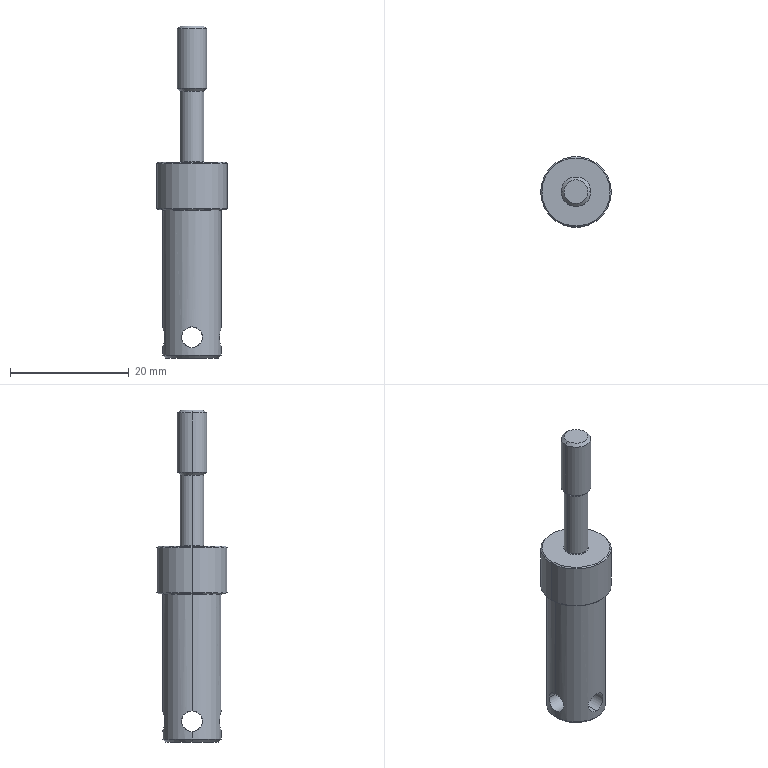Part | SolidWorks | features ICE 5, Chamfer 2, CirPattern 1, Extrusion 1, Fillet 1 | 1 solid | 34 faces | box 11.9 x 11.9 x 56 mm | volume 3013 mm3 | cylinder 16 | cone 10 | torus 4 | plane 4 | commonest cylinder face diameters 3.5 x8 4 x2 5 x2 9.9 x2 11.9 x2
STEP:
#1=CARTESIAN_POINT('',(-4.63,-1.75,-9.));
#2=VERTEX_POINT('',#1);
#3=CARTESIAN_POINT('',(-4.95,0.,-10.75));
#4=VERTEX_POINT('',#3);
#5=CARTESIAN_POINT('',(-4.63,-1.75,-9.));
#6=CARTESIAN_POINT('',(-4.63,-1.75,-9.115));
#7=CARTESIAN_POINT('',(-4.635,-1.738,-9.232));
#8=CARTESIAN_POINT('',(-4.652,-1.693,-9.457));
#9=CARTESIAN_POINT('',(-4.664,-1.66,-9.567));
#10=CARTESIAN_POINT('',(-4.694,-1.571,-9.78));
#11=CARTESIAN_POINT('',(-4.712,-1.517,-9.88));
#12=CARTESIAN_POINT('',(-4.751,-1.39,-10.069));
#13=CARTESIAN_POINT('',(-4.772,-1.317,-10.158));
#14=CARTESIAN_POINT('',(-4.814,-1.156,-10.319));
#15=CARTESIAN_POINT('',(-4.834,-1.069,-10.39));
#16=CARTESIAN_POINT('',(-4.872,-0.8798,-10.517));
#17=CARTESIAN_POINT('',(-4.89,-0.7775,-10.572));
#18=CARTESIAN_POINT('',(-4.933,-0.4616,-10.703));
#19=CARTESIAN_POINT('',(-4.95,-0.2297,-10.75));
#20=CARTESIAN_POINT('',(-4.95,0.,-10.75));
#21=B_SPLINE_CURVE_WITH_KNOTS('',3,(#5,#6,#7,#8,#9,#10,#11,#12,#13,#14,#15,#16,#17,#18,#19,#20),.UNSPECIFIED.,.F.,.F.,(4,2,2,2,2,2,2,4),(0.002759,0.003104,0.003448,0.003793,0.004138,0.004482,0.004827,0.005516),.UNSPECIFIED.);
#22=EDGE_CURVE('',#2,#4,#21,.T.);
#23=ORIENTED_EDGE('',*,*,#22,.F.);
#24=CARTESIAN_POINT('',(-1.75,-1.75,-9.));
#25=VERTEX_POINT('',#24);
#26=CARTESIAN_POINT('',(-8.5,-1.75,-9.));
#27=DIRECTION('',(1.,0.,0.));
#28=VECTOR('',#27,1000.);
#29=LINE('',#26,#28);
#30=EDGE_CURVE('',#2,#25,#29,.T.);
#31=ORIENTED_EDGE('',*,*,#30,.T.);
#32=CARTESIAN_POINT('',(0.,0.,-10.75));
#33=VERTEX_POINT('',#32);
#34=CARTESIAN_POINT('',(0.,0.,-10.75));
#35=CARTESIAN_POINT('',(-1.025,-1.025,-10.75));
#36=CARTESIAN_POINT('',(-1.75,-1.75,-10.025));
#37=CARTESIAN_POINT('',(-1.75,-1.75,-9.));
#38=(BOUNDED_CURVE()B_SPLINE_CURVE(3,(#34,#35,#36,#37),.UNSPECIFIED.,.F.,.F.)B_SPLINE_CURVE_WITH_KNOTS((4,4),(1.571,3.142),.UNSPECIFIED.)CURVE()GEOMETRIC_REPRESENTATION_ITEM()RATIONAL_B_SPLINE_CURVE((1.,0.8047,0.8047,1.))REPRESENTATION_ITEM(''));
#39=EDGE_CURVE('',#33,#25,#38,.T.);
#40=ORIENTED_EDGE('',*,*,#39,.F.);
#41=CARTESIAN_POINT('',(-1.75,1.75,-9.));
#42=VERTEX_POINT('',#41);
#43=CARTESIAN_POINT('',(-1.75,1.75,-9.));
#44=CARTESIAN_POINT('',(-1.75,1.75,-10.025));
#45=CARTESIAN_POINT('',(-1.025,1.025,-10.75));
#46=CARTESIAN_POINT('',(0.,0.,-10.75));
#47=(BOUNDED_CURVE()B_SPLINE_CURVE(3,(#43,#44,#45,#46),.UNSPECIFIED.,.F.,.F.)B_SPLINE_CURVE_WITH_KNOTS((4,4),(0.,1.571),.UNSPECIFIED.)CURVE()GEOMETRIC_REPRESENTATION_ITEM()RATIONAL_B_SPLINE_CURVE((1.,0.8047,0.8047,1.))REPRESENTATION_ITEM(''));
#48=EDGE_CURVE('',#42,#33,#47,.T.);
#49=ORIENTED_EDGE('',*,*,#48,.F.);
#50=CARTESIAN_POINT('',(-4.63,1.75,-9.));
#51=VERTEX_POINT('',#50);
#52=CARTESIAN_POINT('',(-8.5,1.75,-9.));
#53=DIRECTION('',(1.,0.,0.));
#54=VECTOR('',#53,1000.);
#55=LINE('',#52,#54);
#56=EDGE_CURVE('',#51,#42,#55,.T.);
#57=ORIENTED_EDGE('',*,*,#56,.F.);
#58=CARTESIAN_POINT('',(-4.95,0.,-10.75));
#59=CARTESIAN_POINT('',(-4.95,0.2297,-10.75));
#60=CARTESIAN_POINT('',(-4.933,0.4615,-10.704));
#61=CARTESIAN_POINT('',(-4.89,0.7784,-10.572));
#62=CARTESIAN_POINT('',(-4.872,0.8807,-10.517));
#63=CARTESIAN_POINT('',(-4.834,1.069,-10.39));
#64=CARTESIAN_POINT('',(-4.814,1.157,-10.318));
#65=CARTESIAN_POINT('',(-4.751,1.399,-10.075));
#66=CARTESIAN_POINT('',(-4.709,1.527,-9.885));
#67=CARTESIAN_POINT('',(-4.664,1.66,-9.566));
#68=CARTESIAN_POINT('',(-4.651,1.693,-9.457));
#69=CARTESIAN_POINT('',(-4.635,1.738,-9.232));
#70=CARTESIAN_POINT('',(-4.63,1.75,-9.115));
#71=CARTESIAN_POINT('',(-4.63,1.75,-9.));
#72=B_SPLINE_CURVE_WITH_KNOTS('',3,(#58,#59,#60,#61,#62,#63,#64,#65,#66,#67,#68,#69,#70,#71),.UNSPECIFIED.,.F.,.F.,(4,2,2,2,2,2,4),(0.005516,0.006206,0.00655,0.006895,0.007584,0.007929,0.008273),.UNSPECIFIED.);
#73=EDGE_CURVE('',#4,#51,#72,.T.);
#74=ORIENTED_EDGE('',*,*,#73,.F.);
#75=EDGE_LOOP('',(#23,#31,#40,#49,#57,#74));
#76=FACE_OUTER_BOUND('',#75,.T.);
#77=CARTESIAN_POINT('',(-8.5,0.,-9.));
#78=DIRECTION('',(1.,0.,0.));
#79=DIRECTION('',(0.,1.,0.));
#80=AXIS2_PLACEMENT_3D('',#77,#78,#79);
#81=CYLINDRICAL_SURFACE('',#80,1.75);
#82=ADVANCED_FACE('',(#76),#81,.F.);
#83=CARTESIAN_POINT('',(1.75,-1.75,-9.));
#84=VERTEX_POINT('',#83);
#85=CARTESIAN_POINT('',(1.75,-1.75,-9.));
#86=CARTESIAN_POINT('',(1.75,-1.75,-10.025));
#87=CARTESIAN_POINT('',(1.025,-1.025,-10.75));
#88=CARTESIAN_POINT('',(0.,0.,-10.75));
#89=(BOUNDED_CURVE()B_SPLINE_CURVE(3,(#85,#86,#87,#88),.UNSPECIFIED.,.F.,.F.)B_SPLINE_CURVE_WITH_KNOTS((4,4),(3.142,4.712),.UNSPECIFIED.)CURVE()GEOMETRIC_REPRESENTATION_ITEM()RATIONAL_B_SPLINE_CURVE((1.,0.8047,0.8047,1.))REPRESENTATION_ITEM(''));
#90=EDGE_CURVE('',#84,#33,#89,.T.);
#91=ORIENTED_EDGE('',*,*,#90,.F.);
#92=CARTESIAN_POINT('',(4.63,-1.75,-9.));
#93=VERTEX_POINT('',#92);
#94=CARTESIAN_POINT('',(-8.5,-1.75,-9.));
#95=DIRECTION('',(1.,0.,0.));
#96=VECTOR('',#95,1000.);
#97=LINE('',#94,#96);
#98=EDGE_CURVE('',#84,#93,#97,.T.);
#99=ORIENTED_EDGE('',*,*,#98,.T.);
#100=CARTESIAN_POINT('',(4.95,0.,-10.75));
#101=VERTEX_POINT('',#100);
#102=CARTESIAN_POINT('',(4.95,0.,-10.75));
#103=CARTESIAN_POINT('',(4.95,-0.1152,-10.75));
#104=CARTESIAN_POINT('',(4.946,-0.2322,-10.738));
#105=CARTESIAN_POINT('',(4.93,-0.4574,-10.693));
#106=CARTESIAN_POINT('',(4.919,-0.567,-10.66));
#107=CARTESIAN_POINT('',(4.889,-0.7801,-10.571));
#108=CARTESIAN_POINT('',(4.872,-0.8808,-10.516));
#109=CARTESIAN_POINT('',(4.834,-1.069,-10.39));
#110=CARTESIAN_POINT('',(4.813,-1.158,-10.317));
#111=CARTESIAN_POINT('',(4.772,-1.319,-10.156));
#112=CARTESIAN_POINT('',(4.751,-1.391,-10.068));
#113=CARTESIAN_POINT('',(4.712,-1.517,-9.879));
#114=CARTESIAN_POINT('',(4.694,-1.572,-9.777));
#115=CARTESIAN_POINT('',(4.649,-1.703,-9.462));
#116=CARTESIAN_POINT('',(4.63,-1.75,-9.23));
#117=CARTESIAN_POINT('',(4.63,-1.75,-9.));
#118=B_SPLINE_CURVE_WITH_KNOTS('',3,(#102,#103,#104,#105,#106,#107,#108,#109,#110,#111,#112,#113,#114,#115,#116,#117),.UNSPECIFIED.,.F.,.F.,(4,2,2,2,2,2,2,4),(0.002759,0.003104,0.003448,0.003793,0.004137,0.004482,0.004827,0.005516),.UNSPECIFIED.);
#119=EDGE_CURVE('',#101,#93,#118,.T.);
#120=ORIENTED_EDGE('',*,*,#119,.F.);
#121=CARTESIAN_POINT('',(4.63,1.75,-9.));
#122=VERTEX_POINT('',#121);
#123=CARTESIAN_POINT('',(4.63,1.75,-9.));
#124=CARTESIAN_POINT('',(4.63,1.75,-9.117));
#125=CARTESIAN_POINT('',(4.635,1.738,-9.231));
#126=CARTESIAN_POINT('',(4.651,1.693,-9.456));
#127=CARTESIAN_POINT('',(4.664,1.659,-9.568));
#128=CARTESIAN_POINT('',(4.694,1.571,-9.779));
#129=CARTESIAN_POINT('',(4.712,1.517,-9.879));
#130=CARTESIAN_POINT('',(4.751,1.39,-10.069));
#131=CARTESIAN_POINT('',(4.772,1.317,-10.158));
#132=CARTESIAN_POINT('',(4.834,1.077,-10.398));
#133=CARTESIAN_POINT('',(4.875,0.883,-10.528));
#134=CARTESIAN_POINT('',(4.919,0.5674,-10.659));
#135=CARTESIAN_POINT('',(4.93,0.456,-10.693));
#136=CARTESIAN_POINT('',(4.946,0.2295,-10.739));
#137=CARTESIAN_POINT('',(4.95,0.1153,-10.75));
#138=CARTESIAN_POINT('',(4.95,0.,-10.75));
#139=B_SPLINE_CURVE_WITH_KNOTS('',3,(#123,#124,#125,#126,#127,#128,#129,#130,#131,#132,#133,#134,#135,#136,#137,#138),.UNSPECIFIED.,.F.,.F.,(4,2,2,2,2,2,2,4),(0.,0.0003449,0.0006897,0.001035,0.001379,0.002069,0.002414,0.002759),.UNSPECIFIED.);
#140=EDGE_CURVE('',#122,#101,#139,.T.);
#141=ORIENTED_EDGE('',*,*,#140,.F.);
#142=CARTESIAN_POINT('',(1.75,1.75,-9.));
#143=VERTEX_POINT('',#142);
#144=CARTESIAN_POINT('',(-8.5,1.75,-9.));
#145=DIRECTION('',(1.,0.,0.));
#146=VECTOR('',#145,1000.);
#147=LINE('',#144,#146);
#148=EDGE_CURVE('',#143,#122,#147,.T.);
#149=ORIENTED_EDGE('',*,*,#148,.F.);
#150=CARTESIAN_POINT('',(0.,0.,-10.75));
#151=CARTESIAN_POINT('',(1.025,1.025,-10.75));
#152=CARTESIAN_POINT('',(1.75,1.75,-10.025));
#153=CARTESIAN_POINT('',(1.75,1.75,-9.));
#154=(BOUNDED_CURVE()B_SPLINE_CURVE(3,(#150,#151,#152,#153),.UNSPECIFIED.,.F.,.F.)B_SPLINE_CURVE_WITH_KNOTS((4,4),(4.712,6.283),.UNSPECIFIED.)CURVE()GEOMETRIC_REPRESENTATION_ITEM()RATIONAL_B_SPLINE_CURVE((1.,0.8047,0.8047,1.))REPRESENTATION_ITEM(''));
#155=EDGE_CURVE('',#33,#143,#154,.T.);
#156=ORIENTED_EDGE('',*,*,#155,.F.);
#157=EDGE_LOOP('',(#91,#99,#120,#141,#149,#156));
#158=FACE_OUTER_BOUND('',#157,.T.);
#159=CARTESIAN_POINT('',(-8.5,0.,-9.));
#160=DIRECTION('',(1.,0.,0.));
#161=DIRECTION('',(0.,1.,0.));
#162=AXIS2_PLACEMENT_3D('',#159,#160,#161);
#163=CYLINDRICAL_SURFACE('',#162,1.75);
#164=ADVANCED_FACE('',(#158),#163,.F.);
#165=CARTESIAN_POINT('',(0.,-4.95,-10.75));
#166=VERTEX_POINT('',#165);
#167=CARTESIAN_POINT('',(0.,-4.95,-7.25));
#168=VERTEX_POINT('',#167);
#169=CARTESIAN_POINT('',(0.,-4.95,-10.75));
#170=CARTESIAN_POINT('',(-0.2297,-4.95,-10.75));
#171=CARTESIAN_POINT('',(-0.4616,-4.933,-10.703));
#172=CARTESIAN_POINT('',(-0.7785,-4.89,-10.571));
#173=CARTESIAN_POINT('',(-0.8808,-4.872,-10.516));
#174=CARTESIAN_POINT('',(-1.07,-4.834,-10.39));
#175=CARTESIAN_POINT('',(-1.157,-4.814,-10.318));
#176=CARTESIAN_POINT('',(-1.4,-4.751,-10.075));
#177=CARTESIAN_POINT('',(-1.528,-4.709,-9.884));
#178=CARTESIAN_POINT('',(-1.66,-4.664,-9.566));
#179=CARTESIAN_POINT('',(-1.693,-4.651,-9.457));
#180=CARTESIAN_POINT('',(-1.738,-4.635,-9.232));
#181=CARTESIAN_POINT('',(-1.75,-4.63,-9.115));
#182=CARTESIAN_POINT('',(-1.75,-4.63,-8.884));
#183=CARTESIAN_POINT('',(-1.739,-4.635,-8.77));
#184=CARTESIAN_POINT('',(-1.693,-4.651,-8.543));
#185=CARTESIAN_POINT('',(-1.659,-4.664,-8.432));
#186=CARTESIAN_POINT('',(-1.528,-4.709,-8.116));
#187=CARTESIAN_POINT('',(-1.398,-4.751,-7.923));
#188=CARTESIAN_POINT('',(-1.157,-4.814,-7.682));
#189=CARTESIAN_POINT('',(-1.068,-4.834,-7.609));
#190=CARTESIAN_POINT('',(-0.8791,-4.872,-7.483));
#191=CARTESIAN_POINT('',(-0.779,-4.889,-7.429));
#192=CARTESIAN_POINT('',(-0.567,-4.919,-7.34));
#193=CARTESIAN_POINT('',(-0.4557,-4.93,-7.306));
#194=CARTESIAN_POINT('',(-0.2311,-4.946,-7.262));
#195=CARTESIAN_POINT('',(-0.1166,-4.95,-7.25));
#196=CARTESIAN_POINT('',(0.,-4.95,-7.25));
#197=B_SPLINE_CURVE_WITH_KNOTS('',3,(#169,#170,#171,#172,#173,#174,#175,#176,#177,#178,#179,#180,#181,#182,#183,#184,#185,#186,#187,#188,#189,#190,#191,#192,#193,#194,#195,#196),.UNSPECIFIED.,.F.,.F.,(4,2,2,2,2,2,2,2,2,2,2,2,2,4),(0.005516,0.006206,0.00655,0.006895,0.007584,0.007929,0.008274,0.008618,0.008963,0.009652,0.009997,0.01034,0.01069,0.01103),.UNSPECIFIED.);
#198=EDGE_CURVE('',#166,#168,#197,.T.);
#199=ORIENTED_EDGE('',*,*,#198,.F.);
#200=CARTESIAN_POINT('',(0.,-8.5,-10.75));
#201=DIRECTION('',(0.,1.,0.));
#202=VECTOR('',#201,1000.);
#203=LINE('',#200,#202);
#204=EDGE_CURVE('',#166,#33,#203,.T.);
#205=ORIENTED_EDGE('',*,*,#204,.T.);
#206=ORIENTED_EDGE('',*,*,#39,.T.);
#207=CARTESIAN_POINT('',(0.,0.,-7.25));
#208=VERTEX_POINT('',#207);
#209=CARTESIAN_POINT('',(-1.75,-1.75,-9.));
#210=CARTESIAN_POINT('',(-1.75,-1.75,-7.975));
#211=CARTESIAN_POINT('',(-1.025,-1.025,-7.25));
#212=CARTESIAN_POINT('',(0.,0.,-7.25));
#213=(BOUNDED_CURVE()B_SPLINE_CURVE(3,(#209,#210,#211,#212),.UNSPECIFIED.,.F.,.F.)B_SPLINE_CURVE_WITH_KNOTS((4,4),(3.142,4.712),.UNSPECIFIED.)CURVE()GEOMETRIC_REPRESENTATION_ITEM()RATIONAL_B_SPLINE_CURVE((1.,0.8047,0.8047,1.))REPRESENTATION_ITEM(''));
#214=EDGE_CURVE('',#25,#208,#213,.T.);
#215=ORIENTED_EDGE('',*,*,#214,.T.);
#216=CARTESIAN_POINT('',(0.,-8.5,-7.25));
#217=DIRECTION('',(0.,1.,0.));
#218=VECTOR('',#217,1000.);
#219=LINE('',#216,#218);
#220=EDGE_CURVE('',#168,#208,#219,.T.);
#221=ORIENTED_EDGE('',*,*,#220,.F.);
#222=EDGE_LOOP('',(#199,#205,#206,#215,#221));
#223=FACE_OUTER_BOUND('',#222,.T.);
#224=CARTESIAN_POINT('',(0.,-8.5,-9.));
#225=DIRECTION('',(0.,1.,0.));
#226=DIRECTION('',(0.,0.,1.));
#227=AXIS2_PLACEMENT_3D('',#224,#225,#226);
#228=CYLINDRICAL_SURFACE('',#227,1.75);
#229=ADVANCED_FACE('',(#223),#228,.F.);
#230=CARTESIAN_POINT('',(-5.05,0.,12.5));
#231=VERTEX_POINT('',#230);
#232=CARTESIAN_POINT('',(5.05,0.,12.5));
#233=VERTEX_POINT('',#232);
#234=CARTESIAN_POINT('',(0.,0.,12.5));
#235=DIRECTION('',(0.,0.,1.));
#236=DIRECTION('',(1.,0.,0.));
#237=AXIS2_PLACEMENT_3D('',#234,#235,#236);
#238=CIRCLE('',#237,5.05);
#239=EDGE_CURVE('',#231,#233,#238,.T.);
#240=ORIENTED_EDGE('',*,*,#239,.F.);
#241=CARTESIAN_POINT('',(-4.95,0.,12.4));
#242=VERTEX_POINT('',#241);
#243=CARTESIAN_POINT('',(-5.05,0.,12.4));
#244=DIRECTION('',(0.,1.,0.));
#245=DIRECTION('',(-1.,0.,0.));
#246=AXIS2_PLACEMENT_3D('',#243,#244,#245);
#247=CIRCLE('',#246,0.1);
#248=EDGE_CURVE('',#231,#242,#247,.T.);
#249=ORIENTED_EDGE('',*,*,#248,.T.);
#250=CARTESIAN_POINT('',(4.95,0.,12.4));
#251=VERTEX_POINT('',#250);
#252=CARTESIAN_POINT('',(0.,0.,12.4));
#253=DIRECTION('',(0.,0.,-1.));
#254=DIRECTION('',(1.,0.,0.));
#255=AXIS2_PLACEMENT_3D('',#252,#253,#254);
#256=CIRCLE('',#255,4.95);
#257=EDGE_CURVE('',#251,#242,#256,.T.);
#258=ORIENTED_EDGE('',*,*,#257,.F.);
#259=CARTESIAN_POINT('',(5.05,0.,12.4));
#260=DIRECTION('',(0.,-1.,0.));
#261=DIRECTION('',(0.,0.,-1.));
#262=AXIS2_PLACEMENT_3D('',#259,#260,#261);
#263=CIRCLE('',#262,0.1);
#264=EDGE_CURVE('',#233,#251,#263,.T.);
#265=ORIENTED_EDGE('',*,*,#264,.F.);
#266=EDGE_LOOP('',(#240,#249,#258,#265));
#267=FACE_OUTER_BOUND('',#266,.T.);
#268=CARTESIAN_POINT('',(0.,0.,12.4));
#269=DIRECTION('',(0.,0.,1.));
#270=DIRECTION('',(1.,0.,0.));
#271=AXIS2_PLACEMENT_3D('',#268,#269,#270);
#272=TOROIDAL_SURFACE('',#271,5.05,0.1);
#273=ADVANCED_FACE('',(#267),#272,.F.);
#274=CARTESIAN_POINT('',(-2.,0.,20.6));
#275=VERTEX_POINT('',#274);
#276=CARTESIAN_POINT('',(2.,0.,20.6));
#277=VERTEX_POINT('',#276);
#278=CARTESIAN_POINT('',(0.,0.,20.6));
#279=DIRECTION('',(0.,0.,1.));
#280=DIRECTION('',(1.,0.,0.));
#281=AXIS2_PLACEMENT_3D('',#278,#279,#280);
#282=CIRCLE('',#281,2.);
#283=EDGE_CURVE('',#275,#277,#282,.T.);
#284=ORIENTED_EDGE('',*,*,#283,.F.);
#285=CARTESIAN_POINT('',(-2.1,0.,20.5));
#286=VERTEX_POINT('',#285);
#287=CARTESIAN_POINT('',(-2.1,0.,20.6));
#288=DIRECTION('',(0.,1.,0.));
#289=DIRECTION('',(-1.,0.,0.));
#290=AXIS2_PLACEMENT_3D('',#287,#288,#289);
#291=CIRCLE('',#290,0.1);
#292=EDGE_CURVE('',#275,#286,#291,.T.);
#293=ORIENTED_EDGE('',*,*,#292,.T.);
#294=CARTESIAN_POINT('',(2.1,0.,20.5));
#295=VERTEX_POINT('',#294);
#296=CARTESIAN_POINT('',(0.,0.,20.5));
#297=DIRECTION('',(0.,0.,-1.));
#298=DIRECTION('',(1.,0.,0.));
#299=AXIS2_PLACEMENT_3D('',#296,#297,#298);
#300=CIRCLE('',#299,2.1);
#301=EDGE_CURVE('',#295,#286,#300,.T.);
#302=ORIENTED_EDGE('',*,*,#301,.F.);
#303=CARTESIAN_POINT('',(2.1,0.,20.6));
#304=DIRECTION('',(0.,-1.,0.));
#305=DIRECTION('',(0.,0.,-1.));
#306=AXIS2_PLACEMENT_3D('',#303,#304,#305);
#307=CIRCLE('',#306,0.1);
#308=EDGE_CURVE('',#277,#295,#307,.T.);
#309=ORIENTED_EDGE('',*,*,#308,.F.);
#310=EDGE_LOOP('',(#284,#293,#302,#309));
#311=FACE_OUTER_BOUND('',#310,.T.);
#312=CARTESIAN_POINT('',(0.,0.,20.6));
#313=DIRECTION('',(0.,0.,1.));
#314=DIRECTION('',(1.,0.,0.));
#315=AXIS2_PLACEMENT_3D('',#312,#313,#314);
#316=TOROIDAL_SURFACE('',#315,2.1,0.1);
#317=ADVANCED_FACE('',(#311),#316,.F.);
#318=CARTESIAN_POINT('',(-5.75,0.,12.5));
#319=VERTEX_POINT('',#318);
#320=CARTESIAN_POINT('',(5.75,0.,12.5));
#321=VERTEX_POINT('',#320);
#322=CARTESIAN_POINT('',(0.,0.,12.5));
#323=DIRECTION('',(0.,0.,-1.));
#324=DIRECTION('',(1.,0.,0.));
#325=AXIS2_PLACEMENT_3D('',#322,#323,#324);
#326=CIRCLE('',#325,5.75);
#327=EDGE_CURVE('',#319,#321,#326,.T.);
#328=ORIENTED_EDGE('',*,*,#327,.F.);
#329=CARTESIAN_POINT('',(-5.95,0.,12.7));
#330=VERTEX_POINT('',#329);
#331=CARTESIAN_POINT('',(-5.95,0.,12.7));
#332=DIRECTION('',(-0.7071,0.,0.7071));
#333=VECTOR('',#332,1000.);
#334=LINE('',#331,#333);
#335=EDGE_CURVE('',#319,#330,#334,.T.);
#336=ORIENTED_EDGE('',*,*,#335,.T.);
#337=CARTESIAN_POINT('',(5.95,0.,12.7));
#338=VERTEX_POINT('',#337);
#339=CARTESIAN_POINT('',(0.,0.,12.7));
#340=DIRECTION('',(0.,0.,1.));
#341=DIRECTION('',(1.,0.,0.));
#342=AXIS2_PLACEMENT_3D('',#339,#340,#341);
#343=CIRCLE('',#342,5.95);
#344=EDGE_CURVE('',#338,#330,#343,.T.);
#345=ORIENTED_EDGE('',*,*,#344,.F.);
#346=CARTESIAN_POINT('',(5.95,0.,12.7));
#347=DIRECTION('',(0.7071,0.,0.7071));
#348=VECTOR('',#347,1000.);
#349=LINE('',#346,#348);
#350=EDGE_CURVE('',#321,#338,#349,.T.);
#351=ORIENTED_EDGE('',*,*,#350,.F.);
#352=EDGE_LOOP('',(#328,#336,#345,#351));
#353=FACE_OUTER_BOUND('',#352,.T.);
#354=CARTESIAN_POINT('',(0.,0.,12.7));
#355=DIRECTION('',(0.,0.,1.));
#356=DIRECTION('',(1.,0.,0.));
#357=AXIS2_PLACEMENT_3D('',#354,#355,#356);
#358=CONICAL_SURFACE('',#357,5.95,0.7854);
#359=ADVANCED_FACE('',(#353),#358,.T.);
#360=CARTESIAN_POINT('',(5.75,0.,20.5));
#361=VERTEX_POINT('',#360);
#362=CARTESIAN_POINT('',(-5.75,0.,20.5));
#363=VERTEX_POINT('',#362);
#364=CARTESIAN_POINT('',(0.,0.,20.5));
#365=DIRECTION('',(0.,0.,1.));
#366=DIRECTION('',(1.,0.,0.));
#367=AXIS2_PLACEMENT_3D('',#364,#365,#366);
#368=CIRCLE('',#367,5.75);
#369=EDGE_CURVE('',#361,#363,#368,.T.);
#370=ORIENTED_EDGE('',*,*,#369,.F.);
#371=CARTESIAN_POINT('',(5.95,0.,20.3));
#372=VERTEX_POINT('',#371);
#373=CARTESIAN_POINT('',(5.75,0.,20.5));
#374=DIRECTION('',(0.7071,0.,-0.7071));
#375=VECTOR('',#374,1000.);
#376=LINE('',#373,#375);
#377=EDGE_CURVE('',#361,#372,#376,.T.);
#378=ORIENTED_EDGE('',*,*,#377,.T.);
#379=CARTESIAN_POINT('',(-5.95,0.,20.3));
#380=VERTEX_POINT('',#379);
#381=CARTESIAN_POINT('',(0.,0.,20.3));
#382=DIRECTION('',(0.,0.,-1.));
#383=DIRECTION('',(1.,0.,0.));
#384=AXIS2_PLACEMENT_3D('',#381,#382,#383);
#385=CIRCLE('',#384,5.95);
#386=EDGE_CURVE('',#380,#372,#385,.T.);
#387=ORIENTED_EDGE('',*,*,#386,.F.);
#388=CARTESIAN_POINT('',(-5.75,0.,20.5));
#389=DIRECTION('',(-0.7071,0.,-0.7071));
#390=VECTOR('',#389,1000.);
#391=LINE('',#388,#390);
#392=EDGE_CURVE('',#363,#380,#391,.T.);
#393=ORIENTED_EDGE('',*,*,#392,.F.);
#394=EDGE_LOOP('',(#370,#378,#387,#393));
#395=FACE_OUTER_BOUND('',#394,.T.);
#396=CARTESIAN_POINT('',(0.,0.,20.5));
#397=DIRECTION('',(0.,0.,-1.));
#398=DIRECTION('',(-1.,0.,0.));
#399=AXIS2_PLACEMENT_3D('',#396,#397,#398);
#400=CONICAL_SURFACE('',#399,5.75,0.7854);
#401=ADVANCED_FACE('',(#395),#400,.T.);
#402=CARTESIAN_POINT('',(-4.45,0.,-12.5));
#403=VERTEX_POINT('',#402);
#404=CARTESIAN_POINT('',(4.45,0.,-12.5));
#405=VERTEX_POINT('',#404);
#406=CARTESIAN_POINT('',(0.,0.,-12.5));
#407=DIRECTION('',(0.,0.,-1.));
#408=DIRECTION('',(1.,0.,0.));
#409=AXIS2_PLACEMENT_3D('',#406,#407,#408);
#410=CIRCLE('',#409,4.45);
#411=EDGE_CURVE('',#403,#405,#410,.T.);
#412=ORIENTED_EDGE('',*,*,#411,.F.);
#413=CARTESIAN_POINT('',(-4.95,0.,-12.));
#414=VERTEX_POINT('',#413);
#415=CARTESIAN_POINT('',(-4.95,0.,-12.));
#416=DIRECTION('',(-0.7071,0.,0.7071));
#417=VECTOR('',#416,1000.);
#418=LINE('',#415,#417);
#419=EDGE_CURVE('',#403,#414,#418,.T.);
#420=ORIENTED_EDGE('',*,*,#419,.T.);
#421=CARTESIAN_POINT('',(4.95,0.,-12.));
#422=VERTEX_POINT('',#421);
#423=CARTESIAN_POINT('',(0.,0.,-12.));
#424=DIRECTION('',(0.,0.,1.));
#425=DIRECTION('',(1.,0.,0.));
#426=AXIS2_PLACEMENT_3D('',#423,#424,#425);
#427=CIRCLE('',#426,4.95);
#428=EDGE_CURVE('',#422,#414,#427,.T.);
#429=ORIENTED_EDGE('',*,*,#428,.F.);
#430=CARTESIAN_POINT('',(4.95,0.,-12.));
#431=DIRECTION('',(0.7071,0.,0.7071));
#432=VECTOR('',#431,1000.);
#433=LINE('',#430,#432);
#434=EDGE_CURVE('',#405,#422,#433,.T.);
#435=ORIENTED_EDGE('',*,*,#434,.F.);
#436=EDGE_LOOP('',(#412,#420,#429,#435));
#437=FACE_OUTER_BOUND('',#436,.T.);
#438=CARTESIAN_POINT('',(0.,0.,-12.));
#439=DIRECTION('',(0.,0.,1.));
#440=DIRECTION('',(1.,0.,0.));
#441=AXIS2_PLACEMENT_3D('',#438,#439,#440);
#442=CONICAL_SURFACE('',#441,4.95,0.7854);
#443=ADVANCED_FACE('',(#437),#442,.T.);
#444=CARTESIAN_POINT('',(2.,0.,43.5));
#445=VERTEX_POINT('',#444);
#446=CARTESIAN_POINT('',(-2.,0.,43.5));
#447=VERTEX_POINT('',#446);
#448=CARTESIAN_POINT('',(0.,0.,43.5));
#449=DIRECTION('',(0.,0.,1.));
#450=DIRECTION('',(1.,0.,0.));
#451=AXIS2_PLACEMENT_3D('',#448,#449,#450);
#452=CIRCLE('',#451,2.);
#453=EDGE_CURVE('',#445,#447,#452,.T.);
#454=ORIENTED_EDGE('',*,*,#453,.F.);
#455=CARTESIAN_POINT('',(2.5,0.,43.));
#456=VERTEX_POINT('',#455);
#457=CARTESIAN_POINT('',(2.,0.,43.5));
#458=DIRECTION('',(0.7071,0.,-0.7071));
#459=VECTOR('',#458,1000.);
#460=LINE('',#457,#459);
#461=EDGE_CURVE('',#445,#456,#460,.T.);
#462=ORIENTED_EDGE('',*,*,#461,.T.);
#463=CARTESIAN_POINT('',(-2.5,0.,43.));
#464=VERTEX_POINT('',#463);
#465=CARTESIAN_POINT('',(0.,0.,43.));
#466=DIRECTION('',(0.,0.,-1.));
#467=DIRECTION('',(1.,0.,0.));
#468=AXIS2_PLACEMENT_3D('',#465,#466,#467);
#469=CIRCLE('',#468,2.5);
#470=EDGE_CURVE('',#464,#456,#469,.T.);
#471=ORIENTED_EDGE('',*,*,#470,.F.);
#472=CARTESIAN_POINT('',(-2.,0.,43.5));
#473=DIRECTION('',(-0.7071,0.,-0.7071));
#474=VECTOR('',#473,1000.);
#475=LINE('',#472,#474);
#476=EDGE_CURVE('',#447,#464,#475,.T.);
#477=ORIENTED_EDGE('',*,*,#476,.F.);
#478=EDGE_LOOP('',(#454,#462,#471,#477));
#479=FACE_OUTER_BOUND('',#478,.T.);
#480=CARTESIAN_POINT('',(0.,0.,43.5));
#481=DIRECTION('',(0.,0.,-1.));
#482=DIRECTION('',(-1.,0.,0.));
#483=AXIS2_PLACEMENT_3D('',#480,#481,#482);
#484=CONICAL_SURFACE('',#483,2.,0.7854);
#485=ADVANCED_FACE('',(#479),#484,.T.);
#486=CARTESIAN_POINT('',(2.,0.,32.5));
#487=VERTEX_POINT('',#486);
#488=CARTESIAN_POINT('',(-2.,0.,32.5));
#489=VERTEX_POINT('',#488);
#490=CARTESIAN_POINT('',(0.,0.,32.5));
#491=DIRECTION('',(0.,0.,1.));
#492=DIRECTION('',(1.,0.,0.));
#493=AXIS2_PLACEMENT_3D('',#490,#491,#492);
#494=CIRCLE('',#493,2.);
#495=EDGE_CURVE('',#487,#489,#494,.T.);
#496=ORIENTED_EDGE('',*,*,#495,.T.);
#497=CARTESIAN_POINT('',(-2.5,0.,33.));
#498=VERTEX_POINT('',#497);
#499=CARTESIAN_POINT('',(-2.5,0.,33.));
#500=DIRECTION('',(-0.7071,0.,0.7071));
#501=VECTOR('',#500,1000.);
#502=LINE('',#499,#501);
#503=EDGE_CURVE('',#489,#498,#502,.T.);
#504=ORIENTED_EDGE('',*,*,#503,.T.);
#505=CARTESIAN_POINT('',(2.5,0.,33.));
#506=VERTEX_POINT('',#505);
#507=CARTESIAN_POINT('',(0.,0.,33.));
#508=DIRECTION('',(0.,0.,1.));
#509=DIRECTION('',(1.,0.,0.));
#510=AXIS2_PLACEMENT_3D('',#507,#508,#509);
#511=CIRCLE('',#510,2.5);
#512=EDGE_CURVE('',#506,#498,#511,.T.);
#513=ORIENTED_EDGE('',*,*,#512,.F.);
#514=CARTESIAN_POINT('',(2.5,0.,33.));
#515=DIRECTION('',(0.7071,0.,0.7071));
#516=VECTOR('',#515,1000.);
#517=LINE('',#514,#516);
#518=EDGE_CURVE('',#487,#506,#517,.T.);
#519=ORIENTED_EDGE('',*,*,#518,.F.);
#520=EDGE_LOOP('',(#496,#504,#513,#519));
#521=FACE_OUTER_BOUND('',#520,.T.);
#522=CARTESIAN_POINT('',(0.,0.,33.));
#523=DIRECTION('',(0.,0.,1.));
#524=DIRECTION('',(1.,0.,0.));
#525=AXIS2_PLACEMENT_3D('',#522,#523,#524);
#526=CONICAL_SURFACE('',#525,2.5,0.7854);
#527=ADVANCED_FACE('',(#521),#526,.T.);
#528=ORIENTED_EDGE('',*,*,#470,.T.);
#529=CARTESIAN_POINT('',(2.5,0.,43.5));
#530=DIRECTION('',(0.,0.,-1.));
#531=VECTOR('',#530,1000.);
#532=LINE('',#529,#531);
#533=EDGE_CURVE('',#456,#506,#532,.T.);
#534=ORIENTED_EDGE('',*,*,#533,.T.);
#535=ORIENTED_EDGE('',*,*,#512,.T.);
#536=CARTESIAN_POINT('',(-2.5,0.,43.5));
#537=DIRECTION('',(0.,0.,-1.));
#538=VECTOR('',#537,1000.);
#539=LINE('',#536,#538);
#540=EDGE_CURVE('',#464,#498,#539,.T.);
#541=ORIENTED_EDGE('',*,*,#540,.F.);
#542=EDGE_LOOP('',(#528,#534,#535,#541));
#543=FACE_OUTER_BOUND('',#542,.T.);
#544=CARTESIAN_POINT('',(0.,0.,43.5));
#545=DIRECTION('',(0.,0.,-1.));
#546=DIRECTION('',(-1.,0.,0.));
#547=AXIS2_PLACEMENT_3D('',#544,#545,#546);
#548=CYLINDRICAL_SURFACE('',#547,2.5);
#549=ADVANCED_FACE('',(#543),#548,.T.);
#550=ORIENTED_EDGE('',*,*,#495,.F.);
#551=CARTESIAN_POINT('',(2.,0.,32.5));
#552=DIRECTION('',(0.,0.,-1.));
#553=VECTOR('',#552,1000.);
#554=LINE('',#551,#553);
#555=EDGE_CURVE('',#487,#277,#554,.T.);
#556=ORIENTED_EDGE('',*,*,#555,.T.);
#557=CARTESIAN_POINT('',(0.,0.,20.6));
#558=DIRECTION('',(0.,0.,1.));
#559=DIRECTION('',(1.,0.,0.));
#560=AXIS2_PLACEMENT_3D('',#557,#558,#559);
#561=CIRCLE('',#560,2.);
#562=EDGE_CURVE('',#277,#275,#561,.T.);
#563=ORIENTED_EDGE('',*,*,#562,.T.);
#564=CARTESIAN_POINT('',(-2.,0.,32.5));
#565=DIRECTION('',(0.,0.,-1.));
#566=VECTOR('',#565,1000.);
#567=LINE('',#564,#566);
#568=EDGE_CURVE('',#489,#275,#567,.T.);
#569=ORIENTED_EDGE('',*,*,#568,.F.);
#570=EDGE_LOOP('',(#550,#556,#563,#569));
#571=FACE_OUTER_BOUND('',#570,.T.);
#572=CARTESIAN_POINT('',(0.,0.,32.5));
#573=DIRECTION('',(0.,0.,-1.));
#574=DIRECTION('',(-1.,0.,0.));
#575=AXIS2_PLACEMENT_3D('',#572,#573,#574);
#576=CYLINDRICAL_SURFACE('',#575,2.);
#577=ADVANCED_FACE('',(#571),#576,.T.);
#578=ORIENTED_EDGE('',*,*,#386,.T.);
#579=CARTESIAN_POINT('',(5.95,0.,20.5));
#580=DIRECTION('',(0.,0.,-1.));
#581=VECTOR('',#580,1000.);
#582=LINE('',#579,#581);
#583=EDGE_CURVE('',#372,#338,#582,.T.);
#584=ORIENTED_EDGE('',*,*,#583,.T.);
#585=ORIENTED_EDGE('',*,*,#344,.T.);
#586=CARTESIAN_POINT('',(-5.95,0.,20.5));
#587=DIRECTION('',(0.,0.,-1.));
#588=VECTOR('',#587,1000.);
#589=LINE('',#586,#588);
#590=EDGE_CURVE('',#380,#330,#589,.T.);
#591=ORIENTED_EDGE('',*,*,#590,.F.);
#592=EDGE_LOOP('',(#578,#584,#585,#591));
#593=FACE_OUTER_BOUND('',#592,.T.);
#594=CARTESIAN_POINT('',(0.,0.,20.5));
#595=DIRECTION('',(0.,0.,-1.));
#596=DIRECTION('',(-1.,0.,0.));
#597=AXIS2_PLACEMENT_3D('',#594,#595,#596);
#598=CYLINDRICAL_SURFACE('',#597,5.95);
#599=ADVANCED_FACE('',(#593),#598,.T.);
#600=CARTESIAN_POINT('',(0.,4.95,-7.25));
#601=VERTEX_POINT('',#600);
#602=CARTESIAN_POINT('',(0.,4.95,-10.75));
#603=VERTEX_POINT('',#602);
#604=CARTESIAN_POINT('',(0.,4.95,-7.25));
#605=CARTESIAN_POINT('',(-0.1166,4.95,-7.25));
#606=CARTESIAN_POINT('',(-0.2312,4.946,-7.262));
#607=CARTESIAN_POINT('',(-0.4562,4.93,-7.307));
#608=CARTESIAN_POINT('',(-0.5678,4.918,-7.341));
#609=CARTESIAN_POINT('',(-0.7794,4.889,-7.429));
#610=CARTESIAN_POINT('',(-0.8796,4.872,-7.483));
#611=CARTESIAN_POINT('',(-1.069,4.834,-7.61));
#612=CARTESIAN_POINT('',(-1.158,4.813,-7.683));
#613=CARTESIAN_POINT('',(-1.398,4.751,-7.923));
#614=CARTESIAN_POINT('',(-1.528,4.709,-8.117));
#615=CARTESIAN_POINT('',(-1.659,4.664,-8.432));
#616=CARTESIAN_POINT('',(-1.693,4.651,-8.543));
#617=CARTESIAN_POINT('',(-1.739,4.635,-8.77));
#618=CARTESIAN_POINT('',(-1.75,4.63,-8.884));
#619=CARTESIAN_POINT('',(-1.75,4.63,-9.114));
#620=CARTESIAN_POINT('',(-1.738,4.635,-9.231));
#621=CARTESIAN_POINT('',(-1.693,4.651,-9.457));
#622=CARTESIAN_POINT('',(-1.66,4.664,-9.566));
#623=CARTESIAN_POINT('',(-1.571,4.694,-9.779));
#624=CARTESIAN_POINT('',(-1.517,4.712,-9.88));
#625=CARTESIAN_POINT('',(-1.391,4.751,-10.068));
#626=CARTESIAN_POINT('',(-1.317,4.772,-10.158));
#627=CARTESIAN_POINT('',(-1.157,4.814,-10.318));
#628=CARTESIAN_POINT('',(-1.069,4.834,-10.39));
#629=CARTESIAN_POINT('',(-0.88,4.872,-10.517));
#630=CARTESIAN_POINT('',(-0.7777,4.89,-10.572));
#631=CARTESIAN_POINT('',(-0.4617,4.933,-10.703));
#632=CARTESIAN_POINT('',(-0.2298,4.95,-10.75));
#633=CARTESIAN_POINT('',(0.,4.95,-10.75));
#634=B_SPLINE_CURVE_WITH_KNOTS('',3,(#604,#605,#606,#607,#608,#609,#610,#611,#612,#613,#614,#615,#616,#617,#618,#619,#620,#621,#622,#623,#624,#625,#626,#627,#628,#629,#630,#631,#632,#633),.UNSPECIFIED.,.F.,.F.,(4,2,2,2,2,2,2,2,2,2,2,2,2,2,4),(0.,0.0003448,0.0006895,0.001034,0.001379,0.002069,0.002413,0.002758,0.003103,0.003448,0.003792,0.004137,0.004482,0.004827,0.005516),.UNSPECIFIED.);
#635=EDGE_CURVE('',#601,#603,#634,.T.);
#636=ORIENTED_EDGE('',*,*,#635,.T.);
#637=CARTESIAN_POINT('',(0.,4.95,-10.75));
#638=CARTESIAN_POINT('',(0.2297,4.95,-10.75));
#639=CARTESIAN_POINT('',(0.4616,4.933,-10.703));
#640=CARTESIAN_POINT('',(0.7785,4.89,-10.571));
#641=CARTESIAN_POINT('',(0.8808,4.872,-10.516));
#642=CARTESIAN_POINT('',(1.07,4.834,-10.39));
#643=CARTESIAN_POINT('',(1.157,4.814,-10.318));
#644=CARTESIAN_POINT('',(1.4,4.751,-10.075));
#645=CARTESIAN_POINT('',(1.528,4.709,-9.884));
#646=CARTESIAN_POINT('',(1.66,4.664,-9.566));
#647=CARTESIAN_POINT('',(1.693,4.651,-9.457));
#648=CARTESIAN_POINT('',(1.738,4.635,-9.232));
#649=CARTESIAN_POINT('',(1.75,4.63,-9.115));
#650=CARTESIAN_POINT('',(1.75,4.63,-8.884));
#651=CARTESIAN_POINT('',(1.739,4.635,-8.77));
#652=CARTESIAN_POINT('',(1.693,4.651,-8.543));
#653=CARTESIAN_POINT('',(1.659,4.664,-8.432));
#654=CARTESIAN_POINT('',(1.528,4.709,-8.116));
#655=CARTESIAN_POINT('',(1.398,4.751,-7.923));
#656=CARTESIAN_POINT('',(1.157,4.814,-7.682));
#657=CARTESIAN_POINT('',(1.068,4.834,-7.609));
#658=CARTESIAN_POINT('',(0.8791,4.872,-7.483));
#659=CARTESIAN_POINT('',(0.779,4.889,-7.429));
#660=CARTESIAN_POINT('',(0.567,4.919,-7.34));
#661=CARTESIAN_POINT('',(0.4557,4.93,-7.306));
#662=CARTESIAN_POINT('',(0.2311,4.946,-7.262));
#663=CARTESIAN_POINT('',(0.1166,4.95,-7.25));
#664=CARTESIAN_POINT('',(0.,4.95,-7.25));
#665=B_SPLINE_CURVE_WITH_KNOTS('',3,(#637,#638,#639,#640,#641,#642,#643,#644,#645,#646,#647,#648,#649,#650,#651,#652,#653,#654,#655,#656,#657,#658,#659,#660,#661,#662,#663,#664),.UNSPECIFIED.,.F.,.F.,(4,2,2,2,2,2,2,2,2,2,2,2,2,4),(0.005516,0.006206,0.00655,0.006895,0.007584,0.007929,0.008274,0.008618,0.008963,0.009652,0.009997,0.01034,0.01069,0.01103),.UNSPECIFIED.);
#666=EDGE_CURVE('',#603,#601,#665,.T.);
#667=ORIENTED_EDGE('',*,*,#666,.T.);
#668=EDGE_LOOP('',(#636,#667));
#669=FACE_BOUND('',#668,.T.);
#670=CARTESIAN_POINT('',(0.,0.,12.4));
#671=DIRECTION('',(0.,0.,-1.));
#672=DIRECTION('',(1.,0.,0.));
#673=AXIS2_PLACEMENT_3D('',#670,#671,#672);
#674=CIRCLE('',#673,4.95);
#675=EDGE_CURVE('',#242,#251,#674,.T.);
#676=ORIENTED_EDGE('',*,*,#675,.T.);
#677=CARTESIAN_POINT('',(4.95,0.,-7.25));
#678=VERTEX_POINT('',#677);
#679=CARTESIAN_POINT('',(4.95,0.,12.5));
#680=DIRECTION('',(0.,0.,-1.));
#681=VECTOR('',#680,1000.);
#682=LINE('',#679,#681);
#683=EDGE_CURVE('',#251,#678,#682,.T.);
#684=ORIENTED_EDGE('',*,*,#683,.T.);
#685=CARTESIAN_POINT('',(4.95,0.,-7.25));
#686=CARTESIAN_POINT('',(4.95,0.1153,-7.25));
#687=CARTESIAN_POINT('',(4.946,0.2297,-7.261));
#688=CARTESIAN_POINT('',(4.93,0.4564,-7.307));
#689=CARTESIAN_POINT('',(4.918,0.5676,-7.341));
#690=CARTESIAN_POINT('',(4.875,0.8839,-7.472));
#691=CARTESIAN_POINT('',(4.834,1.077,-7.602));
#692=CARTESIAN_POINT('',(4.772,1.318,-7.843));
#693=CARTESIAN_POINT('',(4.751,1.391,-7.932));
#694=CARTESIAN_POINT('',(4.712,1.518,-8.121));
#695=CARTESIAN_POINT('',(4.694,1.571,-8.221));
#696=CARTESIAN_POINT('',(4.664,1.66,-8.433));
#697=CARTESIAN_POINT('',(4.651,1.694,-8.544));
#698=CARTESIAN_POINT('',(4.635,1.738,-8.769));
#699=CARTESIAN_POINT('',(4.63,1.75,-8.883));
#700=CARTESIAN_POINT('',(4.63,1.75,-9.));
#701=B_SPLINE_CURVE_WITH_KNOTS('',3,(#685,#686,#687,#688,#689,#690,#691,#692,#693,#694,#695,#696,#697,#698,#699,#700),.UNSPECIFIED.,.F.,.F.,(4,2,2,2,2,2,2,4),(0.008273,0.008618,0.008962,0.009652,0.009997,0.01034,0.01069,0.01103),.UNSPECIFIED.);
#702=EDGE_CURVE('',#678,#122,#701,.T.);
#703=ORIENTED_EDGE('',*,*,#702,.T.);
#704=ORIENTED_EDGE('',*,*,#140,.T.);
#705=CARTESIAN_POINT('',(4.95,0.,12.5));
#706=DIRECTION('',(0.,0.,-1.));
#707=VECTOR('',#706,1000.);
#708=LINE('',#705,#707);
#709=EDGE_CURVE('',#101,#422,#708,.T.);
#710=ORIENTED_EDGE('',*,*,#709,.T.);
#711=ORIENTED_EDGE('',*,*,#428,.T.);
#712=CARTESIAN_POINT('',(-4.95,0.,12.5));
#713=DIRECTION('',(0.,0.,-1.));
#714=VECTOR('',#713,1000.);
#715=LINE('',#712,#714);
#716=EDGE_CURVE('',#4,#414,#715,.T.);
#717=ORIENTED_EDGE('',*,*,#716,.F.);
#718=ORIENTED_EDGE('',*,*,#73,.T.);
#719=CARTESIAN_POINT('',(-4.95,0.,-7.25));
#720=VERTEX_POINT('',#719);
#721=CARTESIAN_POINT('',(-4.63,1.75,-9.));
#722=CARTESIAN_POINT('',(-4.63,1.75,-8.885));
#723=CARTESIAN_POINT('',(-4.635,1.739,-8.77));
#724=CARTESIAN_POINT('',(-4.651,1.693,-8.544));
#725=CARTESIAN_POINT('',(-4.664,1.659,-8.433));
#726=CARTESIAN_POINT('',(-4.709,1.528,-8.116));
#727=CARTESIAN_POINT('',(-4.751,1.398,-7.923));
#728=CARTESIAN_POINT('',(-4.814,1.157,-7.682));
#729=CARTESIAN_POINT('',(-4.834,1.068,-7.609));
#730=CARTESIAN_POINT('',(-4.872,0.8792,-7.483));
#731=CARTESIAN_POINT('',(-4.889,0.7791,-7.429));
#732=CARTESIAN_POINT('',(-4.919,0.5671,-7.34));
#733=CARTESIAN_POINT('',(-4.93,0.4557,-7.307));
#734=CARTESIAN_POINT('',(-4.946,0.2311,-7.262));
#735=CARTESIAN_POINT('',(-4.95,0.1166,-7.25));
#736=CARTESIAN_POINT('',(-4.95,0.,-7.25));
#737=B_SPLINE_CURVE_WITH_KNOTS('',3,(#721,#722,#723,#724,#725,#726,#727,#728,#729,#730,#731,#732,#733,#734,#735,#736),.UNSPECIFIED.,.F.,.F.,(4,2,2,2,2,2,2,4),(0.008273,0.008618,0.008963,0.009652,0.009997,0.01034,0.01069,0.01103),.UNSPECIFIED.);
#738=EDGE_CURVE('',#51,#720,#737,.T.);
#739=ORIENTED_EDGE('',*,*,#738,.T.);
#740=CARTESIAN_POINT('',(-4.95,0.,12.5));
#741=DIRECTION('',(0.,0.,-1.));
#742=VECTOR('',#741,1000.);
#743=LINE('',#740,#742);
#744=EDGE_CURVE('',#242,#720,#743,.T.);
#745=ORIENTED_EDGE('',*,*,#744,.F.);
#746=EDGE_LOOP('',(#676,#684,#703,#704,#710,#711,#717,#718,#739,#745));
#747=FACE_OUTER_BOUND('',#746,.T.);
#748=CARTESIAN_POINT('',(0.,0.,12.5));
#749=DIRECTION('',(0.,0.,-1.));
#750=DIRECTION('',(-1.,0.,0.));
#751=AXIS2_PLACEMENT_3D('',#748,#749,#750);
#752=CYLINDRICAL_SURFACE('',#751,4.95);
#753=ADVANCED_FACE('',(#669,#747),#752,.T.);
#754=CARTESIAN_POINT('',(0.,0.,-7.25));
#755=CARTESIAN_POINT('',(-1.025,1.025,-7.25));
#756=CARTESIAN_POINT('',(-1.75,1.75,-7.975));
#757=CARTESIAN_POINT('',(-1.75,1.75,-9.));
#758=(BOUNDED_CURVE()B_SPLINE_CURVE(3,(#754,#755,#756,#757),.UNSPECIFIED.,.F.,.F.)B_SPLINE_CURVE_WITH_KNOTS((4,4),(4.712,6.283),.UNSPECIFIED.)CURVE()GEOMETRIC_REPRESENTATION_ITEM()RATIONAL_B_SPLINE_CURVE((1.,0.8047,0.8047,1.))REPRESENTATION_ITEM(''));
#759=EDGE_CURVE('',#208,#42,#758,.T.);
#760=ORIENTED_EDGE('',*,*,#759,.T.);
#761=ORIENTED_EDGE('',*,*,#48,.T.);
#762=CARTESIAN_POINT('',(0.,-8.5,-10.75));
#763=DIRECTION('',(0.,1.,0.));
#764=VECTOR('',#763,1000.);
#765=LINE('',#762,#764);
#766=EDGE_CURVE('',#33,#603,#765,.T.);
#767=ORIENTED_EDGE('',*,*,#766,.T.);
#768=ORIENTED_EDGE('',*,*,#635,.F.);
#769=CARTESIAN_POINT('',(0.,-8.5,-7.25));
#770=DIRECTION('',(0.,1.,0.));
#771=VECTOR('',#770,1000.);
#772=LINE('',#769,#771);
#773=EDGE_CURVE('',#208,#601,#772,.T.);
#774=ORIENTED_EDGE('',*,*,#773,.F.);
#775=EDGE_LOOP('',(#760,#761,#767,#768,#774));
#776=FACE_OUTER_BOUND('',#775,.T.);
#777=CARTESIAN_POINT('',(0.,-8.5,-9.));
#778=DIRECTION('',(0.,1.,0.));
#779=DIRECTION('',(0.,0.,1.));
#780=AXIS2_PLACEMENT_3D('',#777,#778,#779);
#781=CYLINDRICAL_SURFACE('',#780,1.75);
#782=ADVANCED_FACE('',(#776),#781,.F.);
#783=ORIENTED_EDGE('',*,*,#766,.F.);
#784=ORIENTED_EDGE('',*,*,#155,.T.);
#785=CARTESIAN_POINT('',(1.75,1.75,-9.));
#786=CARTESIAN_POINT('',(1.75,1.75,-7.975));
#787=CARTESIAN_POINT('',(1.025,1.025,-7.25));
#788=CARTESIAN_POINT('',(0.,0.,-7.25));
#789=(BOUNDED_CURVE()B_SPLINE_CURVE(3,(#785,#786,#787,#788),.UNSPECIFIED.,.F.,.F.)B_SPLINE_CURVE_WITH_KNOTS((4,4),(0.,1.571),.UNSPECIFIED.)CURVE()GEOMETRIC_REPRESENTATION_ITEM()RATIONAL_B_SPLINE_CURVE((1.,0.8047,0.8047,1.))REPRESENTATION_ITEM(''));
#790=EDGE_CURVE('',#143,#208,#789,.T.);
#791=ORIENTED_EDGE('',*,*,#790,.T.);
#792=ORIENTED_EDGE('',*,*,#773,.T.);
#793=ORIENTED_EDGE('',*,*,#666,.F.);
#794=EDGE_LOOP('',(#783,#784,#791,#792,#793));
#795=FACE_OUTER_BOUND('',#794,.T.);
#796=CARTESIAN_POINT('',(0.,-8.5,-9.));
#797=DIRECTION('',(0.,1.,0.));
#798=DIRECTION('',(0.,0.,1.));
#799=AXIS2_PLACEMENT_3D('',#796,#797,#798);
#800=CYLINDRICAL_SURFACE('',#799,1.75);
#801=ADVANCED_FACE('',(#795),#800,.F.);
#802=ORIENTED_EDGE('',*,*,#301,.T.);
#803=CARTESIAN_POINT('',(0.,0.,20.5));
#804=DIRECTION('',(0.,0.,-1.));
#805=DIRECTION('',(1.,0.,0.));
#806=AXIS2_PLACEMENT_3D('',#803,#804,#805);
#807=CIRCLE('',#806,2.1);
#808=EDGE_CURVE('',#286,#295,#807,.T.);
#809=ORIENTED_EDGE('',*,*,#808,.T.);
#810=EDGE_LOOP('',(#802,#809));
#811=FACE_BOUND('',#810,.T.);
#812=CARTESIAN_POINT('',(0.,0.,20.5));
#813=DIRECTION('',(0.,0.,1.));
#814=DIRECTION('',(1.,0.,0.));
#815=AXIS2_PLACEMENT_3D('',#812,#813,#814);
#816=CIRCLE('',#815,5.75);
#817=EDGE_CURVE('',#363,#361,#816,.T.);
#818=ORIENTED_EDGE('',*,*,#817,.T.);
#819=ORIENTED_EDGE('',*,*,#369,.T.);
#820=EDGE_LOOP('',(#818,#819));
#821=FACE_OUTER_BOUND('',#820,.T.);
#822=CARTESIAN_POINT('',(0.,0.,20.5));
#823=DIRECTION('',(0.,0.,1.));
#824=DIRECTION('',(1.,0.,0.));
#825=AXIS2_PLACEMENT_3D('',#822,#823,#824);
#826=PLANE('',#825);
#827=ADVANCED_FACE('',(#811,#821),#826,.T.);
#828=ORIENTED_EDGE('',*,*,#683,.F.);
#829=ORIENTED_EDGE('',*,*,#257,.T.);
#830=ORIENTED_EDGE('',*,*,#744,.T.);
#831=CARTESIAN_POINT('',(-4.95,0.,-7.25));
#832=CARTESIAN_POINT('',(-4.95,-0.1167,-7.25));
#833=CARTESIAN_POINT('',(-4.946,-0.2312,-7.262));
#834=CARTESIAN_POINT('',(-4.93,-0.4563,-7.307));
#835=CARTESIAN_POINT('',(-4.918,-0.568,-7.341));
#836=CARTESIAN_POINT('',(-4.889,-0.7796,-7.429));
#837=CARTESIAN_POINT('',(-4.872,-0.8799,-7.483));
#838=CARTESIAN_POINT('',(-4.834,-1.069,-7.61));
#839=CARTESIAN_POINT('',(-4.813,-1.158,-7.683));
#840=CARTESIAN_POINT('',(-4.751,-1.398,-7.924));
#841=CARTESIAN_POINT('',(-4.709,-1.528,-8.117));
#842=CARTESIAN_POINT('',(-4.664,-1.659,-8.433));
#843=CARTESIAN_POINT('',(-4.651,-1.694,-8.544));
#844=CARTESIAN_POINT('',(-4.635,-1.739,-8.771));
#845=CARTESIAN_POINT('',(-4.63,-1.75,-8.885));
#846=CARTESIAN_POINT('',(-4.63,-1.75,-9.));
#847=B_SPLINE_CURVE_WITH_KNOTS('',3,(#831,#832,#833,#834,#835,#836,#837,#838,#839,#840,#841,#842,#843,#844,#845,#846),.UNSPECIFIED.,.F.,.F.,(4,2,2,2,2,2,2,4),(0.,0.0003449,0.0006898,0.001035,0.00138,0.002069,0.002414,0.002759),.UNSPECIFIED.);
#848=EDGE_CURVE('',#720,#2,#847,.T.);
#849=ORIENTED_EDGE('',*,*,#848,.T.);
#850=ORIENTED_EDGE('',*,*,#22,.T.);
#851=ORIENTED_EDGE('',*,*,#716,.T.);
#852=CARTESIAN_POINT('',(0.,0.,-12.));
#853=DIRECTION('',(0.,0.,1.));
#854=DIRECTION('',(1.,0.,0.));
#855=AXIS2_PLACEMENT_3D('',#852,#853,#854);
#856=CIRCLE('',#855,4.95);
#857=EDGE_CURVE('',#414,#422,#856,.T.);
#858=ORIENTED_EDGE('',*,*,#857,.T.);
#859=ORIENTED_EDGE('',*,*,#709,.F.);
#860=ORIENTED_EDGE('',*,*,#119,.T.);
#861=CARTESIAN_POINT('',(4.63,-1.75,-9.));
#862=CARTESIAN_POINT('',(4.63,-1.75,-8.77));
#863=CARTESIAN_POINT('',(4.649,-1.704,-8.539));
#864=CARTESIAN_POINT('',(4.694,-1.572,-8.222));
#865=CARTESIAN_POINT('',(4.712,-1.517,-8.12));
#866=CARTESIAN_POINT('',(4.751,-1.39,-7.931));
#867=CARTESIAN_POINT('',(4.772,-1.318,-7.843));
#868=CARTESIAN_POINT('',(4.835,-1.076,-7.601));
#869=CARTESIAN_POINT('',(4.875,-0.885,-7.473));
#870=CARTESIAN_POINT('',(4.919,-0.5665,-7.34));
#871=CARTESIAN_POINT('',(4.93,-0.4572,-7.307));
#872=CARTESIAN_POINT('',(4.946,-0.2323,-7.262));
#873=CARTESIAN_POINT('',(4.95,-0.1153,-7.25));
#874=CARTESIAN_POINT('',(4.95,0.,-7.25));
#875=B_SPLINE_CURVE_WITH_KNOTS('',3,(#861,#862,#863,#864,#865,#866,#867,#868,#869,#870,#871,#872,#873,#874),.UNSPECIFIED.,.F.,.F.,(4,2,2,2,2,2,4),(0.005516,0.006205,0.00655,0.006895,0.007584,0.007928,0.008273),.UNSPECIFIED.);
#876=EDGE_CURVE('',#93,#678,#875,.T.);
#877=ORIENTED_EDGE('',*,*,#876,.T.);
#878=EDGE_LOOP('',(#828,#829,#830,#849,#850,#851,#858,#859,#860,#877));
#879=FACE_OUTER_BOUND('',#878,.T.);
#880=CARTESIAN_POINT('',(0.,-4.95,-7.25));
#881=CARTESIAN_POINT('',(0.1166,-4.95,-7.25));
#882=CARTESIAN_POINT('',(0.2312,-4.946,-7.262));
#883=CARTESIAN_POINT('',(0.4562,-4.93,-7.307));
#884=CARTESIAN_POINT('',(0.5678,-4.918,-7.341));
#885=CARTESIAN_POINT('',(0.7794,-4.889,-7.429));
#886=CARTESIAN_POINT('',(0.8796,-4.872,-7.483));
#887=CARTESIAN_POINT('',(1.069,-4.834,-7.61));
#888=CARTESIAN_POINT('',(1.158,-4.813,-7.683));
#889=CARTESIAN_POINT('',(1.398,-4.751,-7.923));
#890=CARTESIAN_POINT('',(1.528,-4.709,-8.117));
#891=CARTESIAN_POINT('',(1.659,-4.664,-8.432));
#892=CARTESIAN_POINT('',(1.693,-4.651,-8.543));
#893=CARTESIAN_POINT('',(1.739,-4.635,-8.77));
#894=CARTESIAN_POINT('',(1.75,-4.63,-8.884));
#895=CARTESIAN_POINT('',(1.75,-4.63,-9.114));
#896=CARTESIAN_POINT('',(1.738,-4.635,-9.231));
#897=CARTESIAN_POINT('',(1.693,-4.651,-9.457));
#898=CARTESIAN_POINT('',(1.66,-4.664,-9.566));
#899=CARTESIAN_POINT('',(1.571,-4.694,-9.779));
#900=CARTESIAN_POINT('',(1.517,-4.712,-9.88));
#901=CARTESIAN_POINT('',(1.391,-4.751,-10.068));
#902=CARTESIAN_POINT('',(1.317,-4.772,-10.158));
#903=CARTESIAN_POINT('',(1.157,-4.814,-10.318));
#904=CARTESIAN_POINT('',(1.069,-4.834,-10.39));
#905=CARTESIAN_POINT('',(0.88,-4.872,-10.517));
#906=CARTESIAN_POINT('',(0.7777,-4.89,-10.572));
#907=CARTESIAN_POINT('',(0.4617,-4.933,-10.703));
#908=CARTESIAN_POINT('',(0.2298,-4.95,-10.75));
#909=CARTESIAN_POINT('',(0.,-4.95,-10.75));
#910=B_SPLINE_CURVE_WITH_KNOTS('',3,(#880,#881,#882,#883,#884,#885,#886,#887,#888,#889,#890,#891,#892,#893,#894,#895,#896,#897,#898,#899,#900,#901,#902,#903,#904,#905,#906,#907,#908,#909),.UNSPECIFIED.,.F.,.F.,(4,2,2,2,2,2,2,2,2,2,2,2,2,2,4),(0.,0.0003448,0.0006895,0.001034,0.001379,0.002069,0.002413,0.002758,0.003103,0.003448,0.003792,0.004137,0.004482,0.004827,0.005516),.UNSPECIFIED.);
#911=EDGE_CURVE('',#168,#166,#910,.T.);
#912=ORIENTED_EDGE('',*,*,#911,.T.);
#913=ORIENTED_EDGE('',*,*,#198,.T.);
#914=EDGE_LOOP('',(#912,#913));
#915=FACE_BOUND('',#914,.T.);
#916=CARTESIAN_POINT('',(0.,0.,12.5));
#917=DIRECTION('',(0.,0.,-1.));
#918=DIRECTION('',(-1.,0.,0.));
#919=AXIS2_PLACEMENT_3D('',#916,#917,#918);
#920=CYLINDRICAL_SURFACE('',#919,4.95);
#921=ADVANCED_FACE('',(#879,#915),#920,.T.);
#922=CARTESIAN_POINT('',(0.,0.,-12.5));
#923=DIRECTION('',(0.,0.,-1.));
#924=DIRECTION('',(1.,0.,0.));
#925=AXIS2_PLACEMENT_3D('',#922,#923,#924);
#926=CIRCLE('',#925,4.45);
#927=EDGE_CURVE('',#405,#403,#926,.T.);
#928=ORIENTED_EDGE('',*,*,#927,.T.);
#929=ORIENTED_EDGE('',*,*,#411,.T.);
#930=EDGE_LOOP('',(#928,#929));
#931=FACE_OUTER_BOUND('',#930,.T.);
#932=CARTESIAN_POINT('',(0.,0.,-12.5));
#933=DIRECTION('',(0.,0.,1.));
#934=DIRECTION('',(1.,0.,0.));
#935=AXIS2_PLACEMENT_3D('',#932,#933,#934);
#936=PLANE('',#935);
#937=ADVANCED_FACE('',(#931),#936,.F.);
#938=CARTESIAN_POINT('',(0.,0.,12.5));
#939=DIRECTION('',(0.,0.,1.));
#940=DIRECTION('',(1.,0.,0.));
#941=AXIS2_PLACEMENT_3D('',#938,#939,#940);
#942=CIRCLE('',#941,5.05);
#943=EDGE_CURVE('',#233,#231,#942,.T.);
#944=ORIENTED_EDGE('',*,*,#943,.T.);
#945=ORIENTED_EDGE('',*,*,#239,.T.);
#946=EDGE_LOOP('',(#944,#945));
#947=FACE_BOUND('',#946,.T.);
#948=CARTESIAN_POINT('',(0.,0.,12.5));
#949=DIRECTION('',(0.,0.,-1.));
#950=DIRECTION('',(1.,0.,0.));
#951=AXIS2_PLACEMENT_3D('',#948,#949,#950);
#952=CIRCLE('',#951,5.75);
#953=EDGE_CURVE('',#321,#319,#952,.T.);
#954=ORIENTED_EDGE('',*,*,#953,.T.);
#955=ORIENTED_EDGE('',*,*,#327,.T.);
#956=EDGE_LOOP('',(#954,#955));
#957=FACE_OUTER_BOUND('',#956,.T.);
#958=CARTESIAN_POINT('',(0.,0.,12.5));
#959=DIRECTION('',(0.,0.,1.));
#960=DIRECTION('',(1.,0.,0.));
#961=AXIS2_PLACEMENT_3D('',#958,#959,#960);
#962=PLANE('',#961);
#963=ADVANCED_FACE('',(#947,#957),#962,.F.);
#964=ORIENTED_EDGE('',*,*,#583,.F.);
#965=CARTESIAN_POINT('',(0.,0.,20.3));
#966=DIRECTION('',(0.,0.,-1.));
#967=DIRECTION('',(1.,0.,0.));
#968=AXIS2_PLACEMENT_3D('',#965,#966,#967);
#969=CIRCLE('',#968,5.95);
#970=EDGE_CURVE('',#372,#380,#969,.T.);
#971=ORIENTED_EDGE('',*,*,#970,.T.);
#972=ORIENTED_EDGE('',*,*,#590,.T.);
#973=CARTESIAN_POINT('',(0.,0.,12.7));
#974=DIRECTION('',(0.,0.,1.));
#975=DIRECTION('',(1.,0.,0.));
#976=AXIS2_PLACEMENT_3D('',#973,#974,#975);
#977=CIRCLE('',#976,5.95);
#978=EDGE_CURVE('',#330,#338,#977,.T.);
#979=ORIENTED_EDGE('',*,*,#978,.T.);
#980=EDGE_LOOP('',(#964,#971,#972,#979));
#981=FACE_OUTER_BOUND('',#980,.T.);
#982=CARTESIAN_POINT('',(0.,0.,20.5));
#983=DIRECTION('',(0.,0.,-1.));
#984=DIRECTION('',(-1.,0.,0.));
#985=AXIS2_PLACEMENT_3D('',#982,#983,#984);
#986=CYLINDRICAL_SURFACE('',#985,5.95);
#987=ADVANCED_FACE('',(#981),#986,.T.);
#988=ORIENTED_EDGE('',*,*,#555,.F.);
#989=CARTESIAN_POINT('',(0.,0.,32.5));
#990=DIRECTION('',(0.,0.,1.));
#991=DIRECTION('',(1.,0.,0.));
#992=AXIS2_PLACEMENT_3D('',#989,#990,#991);
#993=CIRCLE('',#992,2.);
#994=EDGE_CURVE('',#489,#487,#993,.T.);
#995=ORIENTED_EDGE('',*,*,#994,.F.);
#996=ORIENTED_EDGE('',*,*,#568,.T.);
#997=ORIENTED_EDGE('',*,*,#283,.T.);
#998=EDGE_LOOP('',(#988,#995,#996,#997));
#999=FACE_OUTER_BOUND('',#998,.T.);
#1000=CARTESIAN_POINT('',(0.,0.,32.5));
#1001=DIRECTION('',(0.,0.,-1.));
#1002=DIRECTION('',(-1.,0.,0.));
#1003=AXIS2_PLACEMENT_3D('',#1000,#1001,#1002);
#1004=CYLINDRICAL_SURFACE('',#1003,2.);
#1005=ADVANCED_FACE('',(#999),#1004,.T.);
#1006=ORIENTED_EDGE('',*,*,#533,.F.);
#1007=CARTESIAN_POINT('',(0.,0.,43.));
#1008=DIRECTION('',(0.,0.,-1.));
#1009=DIRECTION('',(1.,0.,0.));
#1010=AXIS2_PLACEMENT_3D('',#1007,#1008,#1009);
#1011=CIRCLE('',#1010,2.5);
#1012=EDGE_CURVE('',#456,#464,#1011,.T.);
#1013=ORIENTED_EDGE('',*,*,#1012,.T.);
#1014=ORIENTED_EDGE('',*,*,#540,.T.);
#1015=CARTESIAN_POINT('',(0.,0.,33.));
#1016=DIRECTION('',(0.,0.,1.));
#1017=DIRECTION('',(1.,0.,0.));
#1018=AXIS2_PLACEMENT_3D('',#1015,#1016,#1017);
#1019=CIRCLE('',#1018,2.5);
#1020=EDGE_CURVE('',#498,#506,#1019,.T.);
#1021=ORIENTED_EDGE('',*,*,#1020,.T.);
#1022=EDGE_LOOP('',(#1006,#1013,#1014,#1021));
#1023=FACE_OUTER_BOUND('',#1022,.T.);
#1024=CARTESIAN_POINT('',(0.,0.,43.5));
#1025=DIRECTION('',(0.,0.,-1.));
#1026=DIRECTION('',(-1.,0.,0.));
#1027=AXIS2_PLACEMENT_3D('',#1024,#1025,#1026);
#1028=CYLINDRICAL_SURFACE('',#1027,2.5);
#1029=ADVANCED_FACE('',(#1023),#1028,.T.);
#1030=CARTESIAN_POINT('',(0.,0.,43.5));
#1031=DIRECTION('',(0.,0.,1.));
#1032=DIRECTION('',(1.,0.,0.));
#1033=AXIS2_PLACEMENT_3D('',#1030,#1031,#1032);
#1034=CIRCLE('',#1033,2.);
#1035=EDGE_CURVE('',#447,#445,#1034,.T.);
#1036=ORIENTED_EDGE('',*,*,#1035,.T.);
#1037=ORIENTED_EDGE('',*,*,#453,.T.);
#1038=EDGE_LOOP('',(#1036,#1037));
#1039=FACE_OUTER_BOUND('',#1038,.T.);
#1040=CARTESIAN_POINT('',(0.,0.,43.5));
#1041=DIRECTION('',(0.,0.,1.));
#1042=DIRECTION('',(1.,0.,0.));
#1043=AXIS2_PLACEMENT_3D('',#1040,#1041,#1042);
#1044=PLANE('',#1043);
#1045=ADVANCED_FACE('',(#1039),#1044,.T.);
#1046=ORIENTED_EDGE('',*,*,#503,.F.);
#1047=ORIENTED_EDGE('',*,*,#994,.T.);
#1048=ORIENTED_EDGE('',*,*,#518,.T.);
#1049=ORIENTED_EDGE('',*,*,#1020,.F.);
#1050=EDGE_LOOP('',(#1046,#1047,#1048,#1049));
#1051=FACE_OUTER_BOUND('',#1050,.T.);
#1052=CARTESIAN_POINT('',(0.,0.,33.));
#1053=DIRECTION('',(0.,0.,1.));
#1054=DIRECTION('',(1.,0.,0.));
#1055=AXIS2_PLACEMENT_3D('',#1052,#1053,#1054);
#1056=CONICAL_SURFACE('',#1055,2.5,0.7854);
#1057=ADVANCED_FACE('',(#1051),#1056,.T.);
#1058=ORIENTED_EDGE('',*,*,#461,.F.);
#1059=ORIENTED_EDGE('',*,*,#1035,.F.);
#1060=ORIENTED_EDGE('',*,*,#476,.T.);
#1061=ORIENTED_EDGE('',*,*,#1012,.F.);
#1062=EDGE_LOOP('',(#1058,#1059,#1060,#1061));
#1063=FACE_OUTER_BOUND('',#1062,.T.);
#1064=CARTESIAN_POINT('',(0.,0.,43.5));
#1065=DIRECTION('',(0.,0.,-1.));
#1066=DIRECTION('',(-1.,0.,0.));
#1067=AXIS2_PLACEMENT_3D('',#1064,#1065,#1066);
#1068=CONICAL_SURFACE('',#1067,2.,0.7854);
#1069=ADVANCED_FACE('',(#1063),#1068,.T.);
#1070=ORIENTED_EDGE('',*,*,#419,.F.);
#1071=ORIENTED_EDGE('',*,*,#927,.F.);
#1072=ORIENTED_EDGE('',*,*,#434,.T.);
#1073=ORIENTED_EDGE('',*,*,#857,.F.);
#1074=EDGE_LOOP('',(#1070,#1071,#1072,#1073));
#1075=FACE_OUTER_BOUND('',#1074,.T.);
#1076=CARTESIAN_POINT('',(0.,0.,-12.));
#1077=DIRECTION('',(0.,0.,1.));
#1078=DIRECTION('',(1.,0.,0.));
#1079=AXIS2_PLACEMENT_3D('',#1076,#1077,#1078);
#1080=CONICAL_SURFACE('',#1079,4.95,0.7854);
#1081=ADVANCED_FACE('',(#1075),#1080,.T.);
#1082=ORIENTED_EDGE('',*,*,#377,.F.);
#1083=ORIENTED_EDGE('',*,*,#817,.F.);
#1084=ORIENTED_EDGE('',*,*,#392,.T.);
#1085=ORIENTED_EDGE('',*,*,#970,.F.);
#1086=EDGE_LOOP('',(#1082,#1083,#1084,#1085));
#1087=FACE_OUTER_BOUND('',#1086,.T.);
#1088=CARTESIAN_POINT('',(0.,0.,20.5));
#1089=DIRECTION('',(0.,0.,-1.));
#1090=DIRECTION('',(-1.,0.,0.));
#1091=AXIS2_PLACEMENT_3D('',#1088,#1089,#1090);
#1092=CONICAL_SURFACE('',#1091,5.75,0.7854);
#1093=ADVANCED_FACE('',(#1087),#1092,.T.);
#1094=ORIENTED_EDGE('',*,*,#335,.F.);
#1095=ORIENTED_EDGE('',*,*,#953,.F.);
#1096=ORIENTED_EDGE('',*,*,#350,.T.);
#1097=ORIENTED_EDGE('',*,*,#978,.F.);
#1098=EDGE_LOOP('',(#1094,#1095,#1096,#1097));
#1099=FACE_OUTER_BOUND('',#1098,.T.);
#1100=CARTESIAN_POINT('',(0.,0.,12.7));
#1101=DIRECTION('',(0.,0.,1.));
#1102=DIRECTION('',(1.,0.,0.));
#1103=AXIS2_PLACEMENT_3D('',#1100,#1101,#1102);
#1104=CONICAL_SURFACE('',#1103,5.95,0.7854);
#1105=ADVANCED_FACE('',(#1099),#1104,.T.);
#1106=ORIENTED_EDGE('',*,*,#292,.F.);
#1107=ORIENTED_EDGE('',*,*,#562,.F.);
#1108=ORIENTED_EDGE('',*,*,#308,.T.);
#1109=ORIENTED_EDGE('',*,*,#808,.F.);
#1110=EDGE_LOOP('',(#1106,#1107,#1108,#1109));
#1111=FACE_OUTER_BOUND('',#1110,.T.);
#1112=CARTESIAN_POINT('',(0.,0.,20.6));
#1113=DIRECTION('',(0.,0.,1.));
#1114=DIRECTION('',(1.,0.,0.));
#1115=AXIS2_PLACEMENT_3D('',#1112,#1113,#1114);
#1116=TOROIDAL_SURFACE('',#1115,2.1,0.1);
#1117=ADVANCED_FACE('',(#1111),#1116,.F.);
#1118=ORIENTED_EDGE('',*,*,#248,.F.);
#1119=ORIENTED_EDGE('',*,*,#943,.F.);
#1120=ORIENTED_EDGE('',*,*,#264,.T.);
#1121=ORIENTED_EDGE('',*,*,#675,.F.);
#1122=EDGE_LOOP('',(#1118,#1119,#1120,#1121));
#1123=FACE_OUTER_BOUND('',#1122,.T.);
#1124=CARTESIAN_POINT('',(0.,0.,12.4));
#1125=DIRECTION('',(0.,0.,1.));
#1126=DIRECTION('',(1.,0.,0.));
#1127=AXIS2_PLACEMENT_3D('',#1124,#1125,#1126);
#1128=TOROIDAL_SURFACE('',#1127,5.05,0.1);
#1129=ADVANCED_FACE('',(#1123),#1128,.F.);
#1130=ORIENTED_EDGE('',*,*,#204,.F.);
#1131=ORIENTED_EDGE('',*,*,#911,.F.);
#1132=ORIENTED_EDGE('',*,*,#220,.T.);
#1133=CARTESIAN_POINT('',(0.,0.,-7.25));
#1134=CARTESIAN_POINT('',(1.025,-1.025,-7.25));
#1135=CARTESIAN_POINT('',(1.75,-1.75,-7.975));
#1136=CARTESIAN_POINT('',(1.75,-1.75,-9.));
#1137=(BOUNDED_CURVE()B_SPLINE_CURVE(3,(#1133,#1134,#1135,#1136),.UNSPECIFIED.,.F.,.F.)B_SPLINE_CURVE_WITH_KNOTS((4,4),(1.571,3.142),.UNSPECIFIED.)CURVE()GEOMETRIC_REPRESENTATION_ITEM()RATIONAL_B_SPLINE_CURVE((1.,0.8047,0.8047,1.))REPRESENTATION_ITEM(''));
#1138=EDGE_CURVE('',#208,#84,#1137,.T.);
#1139=ORIENTED_EDGE('',*,*,#1138,.T.);
#1140=ORIENTED_EDGE('',*,*,#90,.T.);
#1141=EDGE_LOOP('',(#1130,#1131,#1132,#1139,#1140));
#1142=FACE_OUTER_BOUND('',#1141,.T.);
#1143=CARTESIAN_POINT('',(0.,-8.5,-9.));
#1144=DIRECTION('',(0.,1.,0.));
#1145=DIRECTION('',(0.,0.,1.));
#1146=AXIS2_PLACEMENT_3D('',#1143,#1144,#1145);
#1147=CYLINDRICAL_SURFACE('',#1146,1.75);
#1148=ADVANCED_FACE('',(#1142),#1147,.F.);
#1149=ORIENTED_EDGE('',*,*,#98,.F.);
#1150=ORIENTED_EDGE('',*,*,#1138,.F.);
#1151=ORIENTED_EDGE('',*,*,#790,.F.);
#1152=ORIENTED_EDGE('',*,*,#148,.T.);
#1153=ORIENTED_EDGE('',*,*,#702,.F.);
#1154=ORIENTED_EDGE('',*,*,#876,.F.);
#1155=EDGE_LOOP('',(#1149,#1150,#1151,#1152,#1153,#1154));
#1156=FACE_OUTER_BOUND('',#1155,.T.);
#1157=CARTESIAN_POINT('',(-8.5,0.,-9.));
#1158=DIRECTION('',(1.,0.,0.));
#1159=DIRECTION('',(0.,1.,0.));
#1160=AXIS2_PLACEMENT_3D('',#1157,#1158,#1159);
#1161=CYLINDRICAL_SURFACE('',#1160,1.75);
#1162=ADVANCED_FACE('',(#1156),#1161,.F.);
#1163=ORIENTED_EDGE('',*,*,#30,.F.);
#1164=ORIENTED_EDGE('',*,*,#848,.F.);
#1165=ORIENTED_EDGE('',*,*,#738,.F.);
#1166=ORIENTED_EDGE('',*,*,#56,.T.);
#1167=ORIENTED_EDGE('',*,*,#759,.F.);
#1168=ORIENTED_EDGE('',*,*,#214,.F.);
#1169=EDGE_LOOP('',(#1163,#1164,#1165,#1166,#1167,#1168));
#1170=FACE_OUTER_BOUND('',#1169,.T.);
#1171=CARTESIAN_POINT('',(-8.5,0.,-9.));
#1172=DIRECTION('',(1.,0.,0.));
#1173=DIRECTION('',(0.,1.,0.));
#1174=AXIS2_PLACEMENT_3D('',#1171,#1172,#1173);
#1175=CYLINDRICAL_SURFACE('',#1174,1.75);
#1176=ADVANCED_FACE('',(#1170),#1175,.F.);
#1177=CLOSED_SHELL('',(#82,#164,#229,#273,#317,#359,#401,#443,#485,#527,#549,#577,#599,#753,#782,#801,#827,#921,#937,#963,#987,#1005,#1029,#1045,#1057,#1069,#1081,#1093,#1105,#1117,#1129,#1148,#1162,#1176));
#1178=MANIFOLD_SOLID_BREP('',#1177);
#1179=CARTESIAN_POINT('',(0.,0.,0.));
#1180=DIRECTION('',(0.,0.,1.));
#1181=DIRECTION('',(1.,0.,0.));
#1182=AXIS2_PLACEMENT_3D('',#1179,#1180,#1181);
#1183=(LENGTH_UNIT()NAMED_UNIT(*)SI_UNIT(.MILLI.,.METRE.));
#1184=UNCERTAINTY_MEASURE_WITH_UNIT(LENGTH_MEASURE(0.00001),#1183,'','');
#1185=(NAMED_UNIT(*)PLANE_ANGLE_UNIT()SI_UNIT($,.RADIAN.));
#1186=(NAMED_UNIT(*)SI_UNIT($,.STERADIAN.)SOLID_ANGLE_UNIT());
#1187=(GEOMETRIC_REPRESENTATION_CONTEXT(3)GLOBAL_UNCERTAINTY_ASSIGNED_CONTEXT((#1184))GLOBAL_UNIT_ASSIGNED_CONTEXT((#1183,#1185,#1186))REPRESENTATION_CONTEXT('',''));
#1188=ADVANCED_BREP_SHAPE_REPRESENTATION('',(#1178,#1182),#1187);